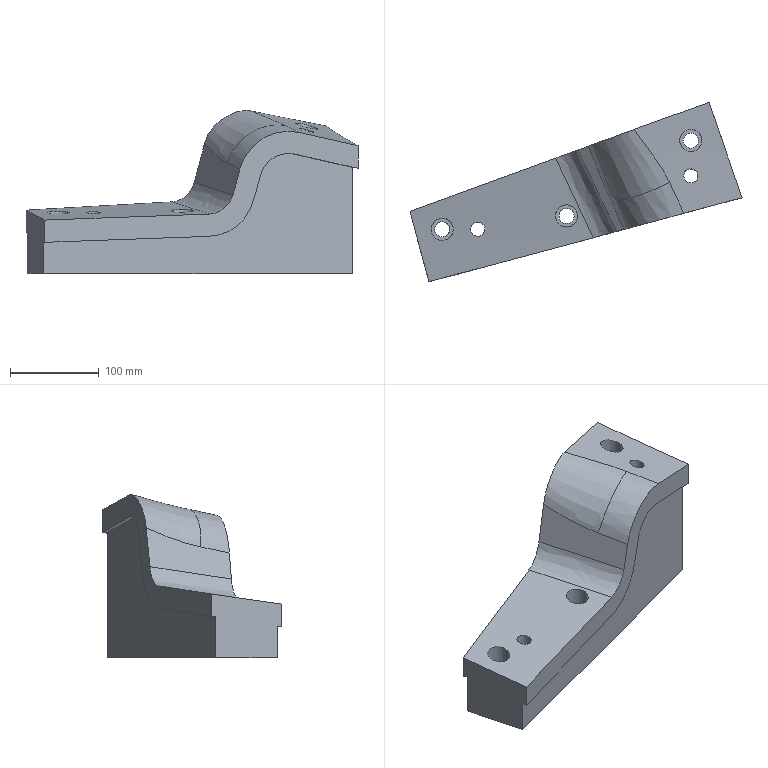Part | NX | features solid 2 | 1 solid | 28 faces | box 373.871 x 202.071 x 183.776 mm | volume 3435387 mm3 | plane 11 | spline 9 | cylinder 8 | commonest cylinder face diameters 17 x3 25 x3 16 x2